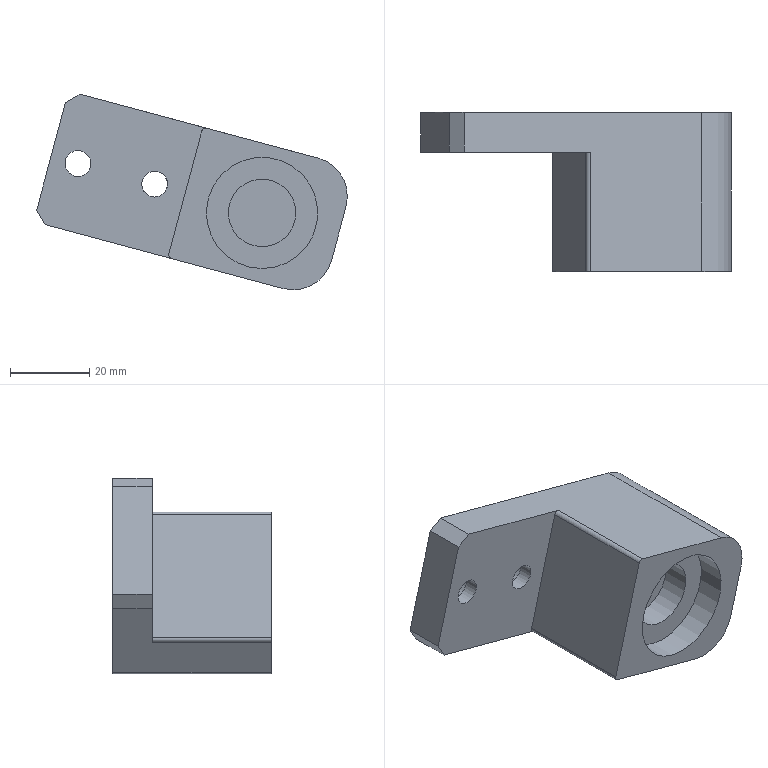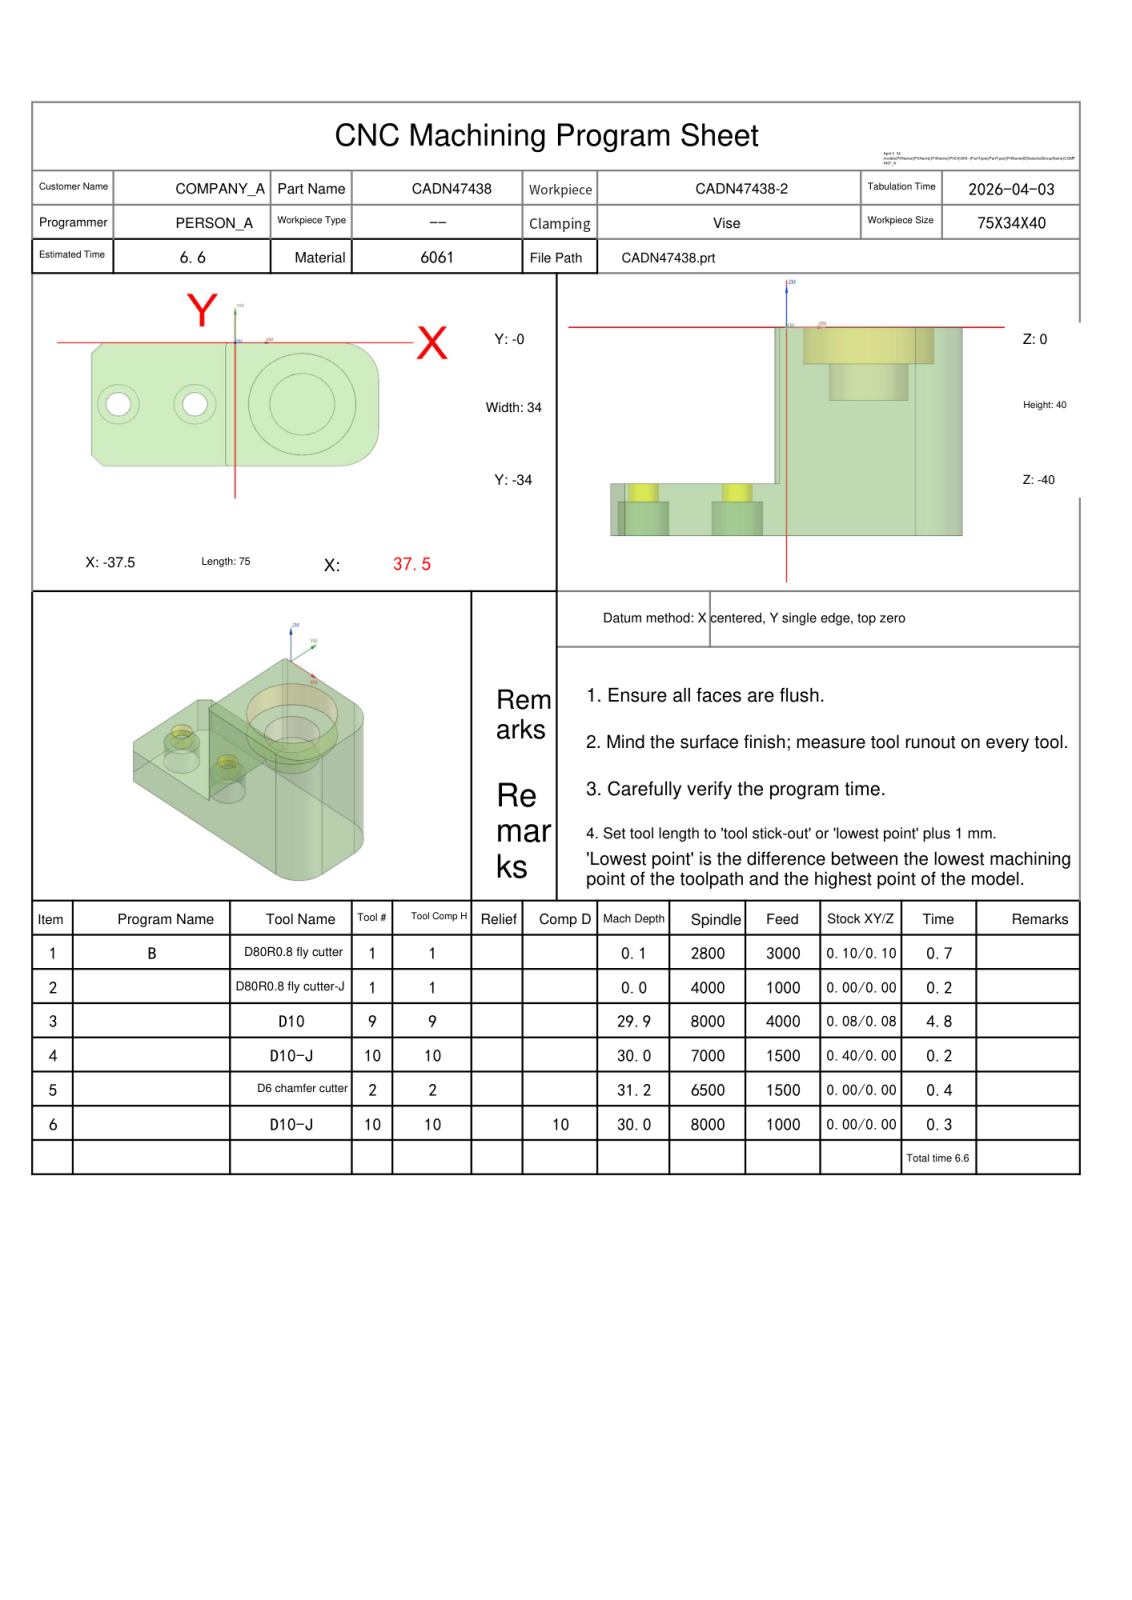NC program | NX | posted by the shop | part box 78.22 x 40 x 49.229 mm
Lines 109 to 1077 of 2756:
N3 T09 M06
(D10  D=10. R=0. H=09 ce=0.08 di=0.08)
G00 G90 G54 X17.5 Y-17. M03 S6000
G43 H09 Z20.
M08
Z.5
G03 X19.432 Y-18.482 I1.932 J.518 F2700.
X21.432 Y-16.482 I0.0 J2.
X21.364 Y-15.965 I-2. J0.0
X21.364 Y-15.965 Z.3 I-3.864 J-1.035 F3000.
X21.364 Y-15.965 Z.1 I-3.864 J-1.035
X21.364 Y-15.965 Z-.1 I-3.864 J-1.035
X21.364 Y-15.965 Z-.3 I-3.864 J-1.035
X21.364 Y-15.965 Z-.5 I-3.864 J-1.035
X21.364 Y-15.965 Z-.7 I-3.864 J-1.035
X21.364 Y-15.965 Z-.9 I-3.864 J-1.035
X21.364 Y-15.965 Z-1.1 I-3.864 J-1.035
X21.364 Y-15.965 Z-1.3 I-3.864 J-1.035
X21.364 Y-15.965 Z-1.5 I-3.864 J-1.035
X21.364 Y-15.965 Z-1.7 I-3.864 J-1.035
X21.364 Y-15.965 Z-1.9 I-3.864 J-1.035
X21.364 Y-15.965 Z-2.1 I-3.864 J-1.035
X21.364 Y-15.965 Z-2.3 I-3.864 J-1.035
X21.364 Y-15.965 Z-2.5 I-3.864 J-1.035
X21.364 Y-15.965 Z-2.7 I-3.864 J-1.035
X21.364 Y-15.965 Z-2.9 I-3.864 J-1.035
X21.364 Y-15.965 Z-3.1 I-3.864 J-1.035
X21.364 Y-15.965 Z-3.3 I-3.864 J-1.035
X21.364 Y-15.965 Z-3.5 I-3.864 J-1.035
X21.364 Y-15.965 Z-3.7 I-3.864 J-1.035
X21.364 Y-15.965 Z-3.9 I-3.864 J-1.035
X21.364 Y-15.965 Z-4.1 I-3.864 J-1.035
X21.364 Y-15.965 Z-4.3 I-3.864 J-1.035
X21.364 Y-15.965 Z-4.5 I-3.864 J-1.035
X21.364 Y-15.965 Z-4.7 I-3.864 J-1.035
X21.364 Y-15.965 Z-4.9 I-3.864 J-1.035
X21.364 Y-15.965 Z-5.1 I-3.864 J-1.035
X21.364 Y-15.965 Z-5.3 I-3.864 J-1.035
X21.364 Y-15.965 Z-5.5 I-3.864 J-1.035
X21.364 Y-15.965 Z-5.7 I-3.864 J-1.035
X21.364 Y-15.965 Z-5.9 I-3.864 J-1.035
X21.364 Y-15.965 Z-6.1 I-3.864 J-1.035
X21.364 Y-15.965 Z-6.3 I-3.864 J-1.035
X21.364 Y-15.965 Z-6.5 I-3.864 J-1.035
X21.364 Y-15.965 Z-6.7 I-3.864 J-1.035
X21.364 Y-15.965 Z-6.9 I-3.864 J-1.035
X20.017 Y-13.891 Z-6.92 I-3.864 J-1.035
X17.445 Y-12.981 I-2.572 J-3.176
X14.319 Y-14.434 I0.0 J-4.087
X13.34 Y-17.116 I3.183 J-2.681
X14.705 Y-20.197 I4.162 J0.0
X17.589 Y-21.311 I2.884 J3.177
X20.713 Y-19.962 I0.0 J4.291
X21.923 Y-16.912 I-3.238 J3.05
X20.583 Y-13.73 I-4.449 J0.0
X17.412 Y-12.438 I-3.171 J-3.246
X14.225 Y-13.746 I0.0 J-4.538
X12.827 Y-17.089 I3.298 J-3.343
X14.12 Y-20.324 I4.696 J0.0
X17.587 Y-21.812 I3.468 J3.297
X20.82 Y-20.555 I0.0 J4.785
X22.423 Y-16.911 I-3.339 J3.644
X21.186 Y-13.639 I-4.943 J0.0
X17.414 Y-11.938 I-3.772 J-3.331
X14.153 Y-13.137 I0.0 J-5.032
X12.326 Y-17.09 I3.363 J-3.953
X13.502 Y-20.379 I5.19 J0.0
X17.585 Y-22.312 I4.084 J3.346
X20.855 Y-21.178 I0.0 J5.279
X22.924 Y-16.91 I-3.367 J4.268
X21.818 Y-13.622 I-5.437 J0.0
X17.416 Y-11.438 I-4.401 J-3.342
X14.157 Y-12.501 I0.0 J-5.526
X11.825 Y-17.091 I3.352 J-4.59
X12.858 Y-20.358 I5.684 J0.0
X17.582 Y-22.813 I4.724 J3.318
X20.812 Y-21.824 I0.0 J5.773
X23.425 Y-16.909 I-3.318 J4.916
X22.471 Y-13.683 I-5.931 J0.0
X17.419 Y-10.937 I-5.051 J-3.275
X14.238 Y-11.846 I0.0 J-6.02
X11.325 Y-17.091 I3.264 J-5.245
X12.197 Y-20.257 I6.178 J0.0
X17.579 Y-23.313 I5.382 J3.212
X20.69 Y-22.486 I0.0 J6.267
X23.926 Y-16.909 I-3.189 J5.577
X23.137 Y-13.824 I-6.425 J0.0
X17.423 Y-10.437 I-5.714 J-3.128
X14.402 Y-11.18 I0.0 J-6.514
X10.824 Y-17.091 I3.094 J-5.911
X11.528 Y-20.074 I6.672 J0.0
X17.576 Y-23.812 I6.048 J3.023
X20.486 Y-23.154 I0.0 J6.761
X24.427 Y-16.909 I-2.978 J6.245
X23.807 Y-14.048 I-6.919 J0.0
X17.426 Y-9.938 I-6.381 J-2.898
X14.648 Y-10.512 I0.0 J-7.008
X10.323 Y-17.091 I2.841 J-6.579
X10.858 Y-19.808 I7.166 J0.0
X17.572 Y-24.312 I6.713 J2.752
X20.197 Y-23.82 I0.0 J7.255
X24.927 Y-16.91 I-2.683 J6.91
X24.474 Y-14.356 I-7.413 J0.0
X17.431 Y-9.438 I-7.043 J-2.584
X14.978 Y-9.85 I0.0 J-7.502
X9.822 Y-17.09 I2.504 J-7.239
X10.197 Y-19.458 I7.66 J0.0
X17.567 Y-24.811 I7.37 J2.396
X19.825 Y-24.475 I0.0 J7.749
X25.428 Y-16.911 I-2.303 J7.564
X25.127 Y-14.749 I-7.907 J0.0
X17.435 Y-8.939 I-7.692 J-2.186
X15.393 Y-9.204 I0.0 J-7.996
X9.322 Y-17.088 I2.082 J-7.883
X9.554 Y-19.022 I8.154 J0.0
X17.562 Y-25.31 I8.008 J1.956
X19.368 Y-25.11 I0.0 J8.243
X25.929 Y-16.913 I-1.84 J8.197
X25.758 Y-15.227 I-8.401 J0.0
X17.44 Y-8.441 I-8.318 J-1.704
X15.892 Y-8.583 I0.0 J-8.49
X8.821 Y-17.086 I1.577 J-8.503
X8.938 Y-18.504 I8.648 J0.0
X17.597 Y-25.842 I8.659 J1.439
X18.949 Y-25.737 I0.0 J8.777
X26.439 Y-16.988 I-1.365 J8.749
X26.357 Y-15.787 I-8.854 J0.0
X17.5 Y-8.06 I-8.857 J-1.213
X8.56 Y-17. I0.0 J-8.94
X17.5 Y-25.94 I8.94 J0.0
X26.44 Y-17. I0.0 J8.94
X26.276 Y-15.293 I-8.94 J0.0
X21.888 Y-11.677 I-4.388 J-.853
X17.418 Y-16.147 I0.0 J-4.47
X17.5 Y-17. I4.47 J0.0
G00 Z20.
G00 G90 X20.279 Y-18.949 M03 S8000
Z20.
Z-6.
G01 X20.47 Y-18.715 Z-6.016 F2000.
X20.864 Y-17.672 Z-6.074
X20.901 Y-16.557 Z-6.133
X20.667 Y-15.683 Z-6.18
X20.077 Y-14.737 Z-6.239
X19.215 Y-14.03 Z-6.297
X18.172 Y-13.636 Z-6.355
X17.057 Y-13.599 Z-6.414
X16.183 Y-13.833 Z-6.461
X15.237 Y-14.423 Z-6.52
X14.53 Y-15.285 Z-6.578
X14.136 Y-16.328 Z-6.637
X14.099 Y-17.443 Z-6.695
X14.333 Y-18.317 Z-6.743
X14.923 Y-19.263 Z-6.801
X15.785 Y-19.97 Z-6.859
X16.828 Y-20.364 Z-6.918
X17.943 Y-20.401 Z-6.976
X18.38 Y-20.284 Z-7.
G03 X20.784 Y-16.12 Z-7.062 I-.88 J3.284
X16.62 Y-13.716 Z-7.123 I-3.284 J-.88
X14.216 Y-17.88 Z-7.185 I.88 J-3.284
X18.38 Y-20.284 Z-7.246 I3.284 J.88
X20.784 Y-16.12 Z-7.308 I-.88 J3.284
X16.62 Y-13.716 Z-7.37 I-3.284 J-.88
X14.216 Y-17.88 Z-7.431 I.88 J-3.284
X18.38 Y-20.284 Z-7.493 I3.284 J.88
X20.784 Y-16.12 Z-7.554 I-.88 J3.284
X16.62 Y-13.716 Z-7.616 I-3.284 J-.88
X14.216 Y-17.88 Z-7.678 I.88 J-3.284
X18.38 Y-20.284 Z-7.739 I3.284 J.88
X20.784 Y-16.12 Z-7.801 I-.88 J3.284
X16.62 Y-13.716 Z-7.863 I-3.284 J-.88
X14.216 Y-17.88 Z-7.924 I.88 J-3.284
X18.38 Y-20.284 Z-7.986 I3.284 J.88
X20.784 Y-16.12 Z-8.047 I-.88 J3.284
X16.62 Y-13.716 Z-8.109 I-3.284 J-.88
X14.216 Y-17.88 Z-8.171 I.88 J-3.284
X18.38 Y-20.284 Z-8.232 I3.284 J.88
X20.784 Y-16.12 Z-8.294 I-.88 J3.284
X16.62 Y-13.716 Z-8.355 I-3.284 J-.88
X14.216 Y-17.88 Z-8.417 I.88 J-3.284
X18.38 Y-20.284 Z-8.479 I3.284 J.88
X20.784 Y-16.12 Z-8.54 I-.88 J3.284
X16.62 Y-13.716 Z-8.602 I-3.284 J-.88
X14.216 Y-17.88 Z-8.663 I.88 J-3.284
X18.38 Y-20.284 Z-8.725 I3.284 J.88
X20.784 Y-16.12 Z-8.787 I-.88 J3.284
X16.62 Y-13.716 Z-8.848 I-3.284 J-.88
X14.216 Y-17.88 Z-8.91 I.88 J-3.284
X18.38 Y-20.284 Z-8.971 I3.284 J.88
X20.784 Y-16.12 Z-9.033 I-.88 J3.284
X16.62 Y-13.716 Z-9.095 I-3.284 J-.88
X14.216 Y-17.88 Z-9.156 I.88 J-3.284
X18.38 Y-20.284 Z-9.218 I3.284 J.88
X20.784 Y-16.12 Z-9.279 I-.88 J3.284
X16.62 Y-13.716 Z-9.341 I-3.284 J-.88
X14.216 Y-17.88 Z-9.403 I.88 J-3.284
X18.38 Y-20.284 Z-9.464 I3.284 J.88
X20.784 Y-16.12 Z-9.526 I-.88 J3.284
X16.62 Y-13.716 Z-9.588 I-3.284 J-.88
X14.216 Y-17.88 Z-9.649 I.88 J-3.284
X18.38 Y-20.284 Z-9.711 I3.284 J.88
X20.784 Y-16.12 Z-9.772 I-.88 J3.284
X16.62 Y-13.716 Z-9.834 I-3.284 J-.88
X14.216 Y-17.88 Z-9.896 I.88 J-3.284
X18.38 Y-20.284 Z-9.957 I3.284 J.88
X20.784 Y-16.12 Z-10.019 I-.88 J3.284
X16.62 Y-13.716 Z-10.08 I-3.284 J-.88
X14.216 Y-17.88 Z-10.142 I.88 J-3.284
X18.38 Y-20.284 Z-10.204 I3.284 J.88
X20.784 Y-16.12 Z-10.265 I-.88 J3.284
X16.62 Y-13.716 Z-10.327 I-3.284 J-.88
X14.216 Y-17.88 Z-10.388 I.88 J-3.284
X18.38 Y-20.284 Z-10.45 I3.284 J.88
X20.784 Y-16.12 Z-10.512 I-.88 J3.284
X16.62 Y-13.716 Z-10.573 I-3.284 J-.88
X14.216 Y-17.88 Z-10.635 I.88 J-3.284
X18.38 Y-20.284 Z-10.696 I3.284 J.88
X20.784 Y-16.12 Z-10.758 I-.88 J3.284
X16.62 Y-13.716 Z-10.82 I-3.284 J-.88
X14.216 Y-17.88 Z-10.881 I.88 J-3.284
X18.38 Y-20.284 Z-10.943 I3.284 J.88
X20.784 Y-16.12 Z-11.004 I-.88 J3.284
X16.62 Y-13.716 Z-11.066 I-3.284 J-.88
X14.216 Y-17.88 Z-11.128 I.88 J-3.284
X18.38 Y-20.284 Z-11.189 I3.284 J.88
X20.784 Y-16.12 Z-11.251 I-.88 J3.284
X16.62 Y-13.716 Z-11.313 I-3.284 J-.88
X14.216 Y-17.88 Z-11.374 I.88 J-3.284
X18.38 Y-20.284 Z-11.436 I3.284 J.88
X20.784 Y-16.12 Z-11.497 I-.88 J3.284
X16.62 Y-13.716 Z-11.559 I-3.284 J-.88
X14.216 Y-17.88 Z-11.621 I.88 J-3.284
X18.38 Y-20.284 Z-11.682 I3.284 J.88
X20.784 Y-16.12 Z-11.744 I-.88 J3.284
X16.62 Y-13.716 Z-11.805 I-3.284 J-.88
X14.216 Y-17.88 Z-11.867 I.88 J-3.284
X18.38 Y-20.284 Z-11.929 I3.284 J.88
X20.784 Y-16.12 Z-11.99 I-.88 J3.284
X16.62 Y-13.716 Z-12.052 I-3.284 J-.88
X14.216 Y-17.88 Z-12.113 I.88 J-3.284
X18.38 Y-20.284 Z-12.175 I3.284 J.88
X20.784 Y-16.12 Z-12.237 I-.88 J3.284
X16.62 Y-13.716 Z-12.298 I-3.284 J-.88
X14.216 Y-17.88 Z-12.36 I.88 J-3.284
X18.38 Y-20.284 Z-12.421 I3.284 J.88
X20.784 Y-16.12 Z-12.483 I-.88 J3.284
X16.62 Y-13.716 Z-12.545 I-3.284 J-.88
X14.216 Y-17.88 Z-12.606 I.88 J-3.284
X18.38 Y-20.284 Z-12.668 I3.284 J.88
X20.784 Y-16.12 Z-12.729 I-.88 J3.284
X16.62 Y-13.716 Z-12.791 I-3.284 J-.88
X14.216 Y-17.88 Z-12.853 I.88 J-3.284
X18.38 Y-20.284 Z-12.914 I3.284 J.88
X20.784 Y-16.12 Z-12.976 I-.88 J3.284
X16.62 Y-13.716 Z-13.038 I-3.284 J-.88
X14.216 Y-17.88 Z-13.099 I.88 J-3.284
X18.38 Y-20.284 Z-13.161 I3.284 J.88
X20.784 Y-16.12 Z-13.222 I-.88 J3.284
X16.62 Y-13.716 Z-13.284 I-3.284 J-.88
X14.216 Y-17.88 Z-13.346 I.88 J-3.284
X18.38 Y-20.284 Z-13.407 I3.284 J.88
X20.784 Y-16.12 Z-13.469 I-.88 J3.284
X16.62 Y-13.716 Z-13.53 I-3.284 J-.88
X14.216 Y-17.88 Z-13.592 I.88 J-3.284
X18.38 Y-20.284 Z-13.654 I3.284 J.88
X20.784 Y-16.12 Z-13.715 I-.88 J3.284
X16.62 Y-13.716 Z-13.777 I-3.284 J-.88
X14.216 Y-17.88 Z-13.838 I.88 J-3.284
X18.38 Y-20.284 Z-13.9 I3.284 J.88
X20.9 Y-17. I-.88 J3.284
X17.5 Y-13.6 I-3.4 J0.0
X14.1 Y-17. I0.0 J-3.4
X17.5 Y-20.4 I3.4 J0.0
X18.38 Y-20.284 I0.0 J3.4
X18.759 Y-20.158 I-.88 J3.284
G01 Z-12.9
G00 Z20.
G00 G90 X-36.67 Y-41.997 M03 S8000
Z14.5
Z.902
G01 Z-.598 F4000.
X-37.222 Y-38.207
G02 X-37.6 Y-33. I35.722 J5.207
G01 Y-1.
G02 X-37.27 Y3.872 I36.1 J0.0
X-36.986 Y4.443 I.991 J-.135
G01 X-36.822 Y4.607
G02 X-36.116 Y4.9 I.707 J-.707
G01 X-30.454
G02 X-29.654 Y4.1 I0.0 J-.8
G01 X-29.666 Y3.962
G03 X-30.1 Y-1. I28.166 J-4.962
G01 Y-33.
G03 X-29.646 Y-38.078 I28.6 J0.0
X-28.662 Y-38.9 I.984 J.178
G01 X-22.67
G03 X-21.971 Y-38.2 I0.0 J.7
G01 X-21.991 Y-38.033
G02 X-22.6 Y-33. I20.491 J5.033
G01 Y-1.
G02 X-21.963 Y4.144 I21.1 J0.0
X-20.994 Y4.9 I.97 J-.244
G01 X-14.673
G02 X-14.074 Y4.3 I0.0 J-.6
X-14.117 Y4.076 I-.6 J0.0
G03 X-15.1 Y-1. I12.617 J-5.076
G01 Y-33.
G03 X-13.977 Y-38.412 I13.6 J0.0
X-13.246 Y-38.996 I.917 J.398
G01 X-3.49 Y-40.85
X-3.303 Y-40.867
G03 X-2.303 Y-39.867 I0.0 J1.
X-3.049 Y-38.9 I-1. J0.0
G02 X-7.6 Y-33. I1.549 J5.9
G01 Y-1.
G02 X-3.049 Y4.9 I6.1 J0.0
G01 X-.148 Y5.662
Y8.1
Z.902
G00 Z14.5
X-36.67 Y-41.997
Z.304
G01 Z-1.196
X-37.222 Y-38.207
G02 X-37.6 Y-33. I35.722 J5.207
G01 Y-1.
G02 X-37.27 Y3.872 I36.1 J0.0
X-36.986 Y4.443 I.991 J-.135
G01 X-36.822 Y4.607
G02 X-36.116 Y4.9 I.707 J-.707
G01 X-30.454
G02 X-29.654 Y4.1 I0.0 J-.8
G01 X-29.666 Y3.962
G03 X-30.1 Y-1. I28.166 J-4.962
G01 Y-33.
G03 X-29.646 Y-38.078 I28.6 J0.0
X-28.662 Y-38.9 I.984 J.178
G01 X-22.67
G03 X-21.971 Y-38.2 I0.0 J.7
G01 X-21.991 Y-38.033
G02 X-22.6 Y-33. I20.491 J5.033
G01 Y-1.
G02 X-21.963 Y4.144 I21.1 J0.0
X-20.994 Y4.9 I.97 J-.244
G01 X-14.673
G02 X-14.074 Y4.3 I0.0 J-.6
X-14.117 Y4.076 I-.6 J0.0
G03 X-15.1 Y-1. I12.617 J-5.076
G01 Y-33.
G03 X-13.977 Y-38.412 I13.6 J0.0
X-13.246 Y-38.996 I.917 J.398
G01 X-3.49 Y-40.85
X-3.303 Y-40.867
G03 X-2.303 Y-39.867 I0.0 J1.
X-3.049 Y-38.9 I-1. J0.0
G02 X-7.6 Y-33. I1.549 J5.9
G01 Y-1.
G02 X-3.049 Y4.9 I6.1 J0.0
G01 X-.148 Y5.662
Y8.1
Z.304
G00 Z14.5
X-36.67 Y-41.997
Z-.294
G01 Z-1.794
X-37.222 Y-38.207
G02 X-37.6 Y-33. I35.722 J5.207
G01 Y-1.
G02 X-37.27 Y3.872 I36.1 J0.0
X-36.986 Y4.443 I.991 J-.135
G01 X-36.822 Y4.607
G02 X-36.116 Y4.9 I.707 J-.707
G01 X-30.454
G02 X-29.654 Y4.1 I0.0 J-.8
G01 X-29.666 Y3.962
G03 X-30.1 Y-1. I28.166 J-4.962
G01 Y-33.
G03 X-29.646 Y-38.078 I28.6 J0.0
X-28.662 Y-38.9 I.984 J.178
G01 X-22.67
G03 X-21.971 Y-38.2 I0.0 J.7
G01 X-21.991 Y-38.033
G02 X-22.6 Y-33. I20.491 J5.033
G01 Y-1.
G02 X-21.963 Y4.144 I21.1 J0.0
X-20.994 Y4.9 I.97 J-.244
G01 X-14.673
G02 X-14.074 Y4.3 I0.0 J-.6
X-14.117 Y4.076 I-.6 J0.0
G03 X-15.1 Y-1. I12.617 J-5.076
G01 Y-33.
G03 X-13.977 Y-38.412 I13.6 J0.0
X-13.246 Y-38.996 I.917 J.398
G01 X-3.49 Y-40.85
X-3.303 Y-40.867
G03 X-2.303 Y-39.867 I0.0 J1.
X-3.049 Y-38.9 I-1. J0.0
G02 X-7.6 Y-33. I1.549 J5.9
G01 Y-1.
G02 X-3.049 Y4.9 I6.1 J0.0
G01 X-.148 Y5.662
Y8.1
Z-.294
G00 Z14.5
X-36.67 Y-41.997
Z-.892
G01 Z-2.392
X-37.222 Y-38.207
G02 X-37.6 Y-33. I35.722 J5.207
G01 Y-1.
G02 X-37.27 Y3.872 I36.1 J0.0
X-36.986 Y4.443 I.991 J-.135
G01 X-36.822 Y4.607
G02 X-36.116 Y4.9 I.707 J-.707
G01 X-30.454
G02 X-29.654 Y4.1 I0.0 J-.8
G01 X-29.666 Y3.962
G03 X-30.1 Y-1. I28.166 J-4.962
G01 Y-33.
G03 X-29.646 Y-38.078 I28.6 J0.0
X-28.662 Y-38.9 I.984 J.178
G01 X-22.67
G03 X-21.971 Y-38.2 I0.0 J.7
G01 X-21.991 Y-38.033
G02 X-22.6 Y-33. I20.491 J5.033
G01 Y-1.
G02 X-21.963 Y4.144 I21.1 J0.0
X-20.994 Y4.9 I.97 J-.244
G01 X-14.673
G02 X-14.074 Y4.3 I0.0 J-.6
X-14.117 Y4.076 I-.6 J0.0
G03 X-15.1 Y-1. I12.617 J-5.076
G01 Y-33.
G03 X-13.977 Y-38.412 I13.6 J0.0
X-13.246 Y-38.996 I.917 J.398
G01 X-3.49 Y-40.85
X-3.303 Y-40.867
G03 X-2.303 Y-39.867 I0.0 J1.
X-3.049 Y-38.9 I-1. J0.0
G02 X-7.6 Y-33. I1.549 J5.9
G01 Y-1.
G02 X-3.049 Y4.9 I6.1 J0.0
G01 X-.148 Y5.662
Y8.1
Z-.892
G00 Z14.5
X-36.67 Y-41.997
Z-1.49
G01 Z-2.99
X-37.222 Y-38.207
G02 X-37.6 Y-33. I35.722 J5.207
G01 Y-1.
G02 X-37.27 Y3.872 I36.1 J0.0
X-36.986 Y4.443 I.991 J-.135
G01 X-36.822 Y4.607
G02 X-36.116 Y4.9 I.707 J-.707
G01 X-30.454
G02 X-29.654 Y4.1 I0.0 J-.8
G01 X-29.666 Y3.962
G03 X-30.1 Y-1. I28.166 J-4.962
G01 Y-33.
G03 X-29.646 Y-38.078 I28.6 J0.0
X-28.662 Y-38.9 I.984 J.178
G01 X-22.67
G03 X-21.971 Y-38.2 I0.0 J.7
G01 X-21.991 Y-38.033
G02 X-22.6 Y-33. I20.491 J5.033
G01 Y-1.
G02 X-21.963 Y4.144 I21.1 J0.0
X-20.994 Y4.9 I.97 J-.244
G01 X-14.673
G02 X-14.074 Y4.3 I0.0 J-.6
X-14.117 Y4.076 I-.6 J0.0
G03 X-15.1 Y-1. I12.617 J-5.076
G01 Y-33.
G03 X-13.977 Y-38.412 I13.6 J0.0
X-13.246 Y-38.996 I.917 J.398
G01 X-3.49 Y-40.85
X-3.303 Y-40.867
G03 X-2.303 Y-39.867 I0.0 J1.
X-3.049 Y-38.9 I-1. J0.0
G02 X-7.6 Y-33. I1.549 J5.9
G01 Y-1.
G02 X-3.049 Y4.9 I6.1 J0.0
G01 X-.148 Y5.662
Y8.1
Z-1.49
G00 Z14.5
X-36.67 Y-41.997
Z-2.088
G01 Z-3.588
X-37.222 Y-38.207
G02 X-37.6 Y-33. I35.722 J5.207
G01 Y-1.
G02 X-37.27 Y3.872 I36.1 J0.0
X-36.986 Y4.443 I.991 J-.135
G01 X-36.822 Y4.607
G02 X-36.116 Y4.9 I.707 J-.707
G01 X-30.454
G02 X-29.654 Y4.1 I0.0 J-.8
G01 X-29.666 Y3.962
G03 X-30.1 Y-1. I28.166 J-4.962
G01 Y-33.
G03 X-29.646 Y-38.078 I28.6 J0.0
X-28.662 Y-38.9 I.984 J.178
G01 X-22.67
G03 X-21.971 Y-38.2 I0.0 J.7
G01 X-21.991 Y-38.033
G02 X-22.6 Y-33. I20.491 J5.033
G01 Y-1.
G02 X-21.963 Y4.144 I21.1 J0.0
X-20.994 Y4.9 I.97 J-.244
G01 X-14.673
G02 X-14.074 Y4.3 I0.0 J-.6
X-14.117 Y4.076 I-.6 J0.0
G03 X-15.1 Y-1. I12.617 J-5.076
G01 Y-33.
G03 X-13.977 Y-38.412 I13.6 J0.0
X-13.246 Y-38.996 I.917 J.398
G01 X-3.49 Y-40.85
X-3.303 Y-40.867
G03 X-2.303 Y-39.867 I0.0 J1.
X-3.049 Y-38.9 I-1. J0.0
G02 X-7.6 Y-33. I1.549 J5.9
G01 Y-1.
G02 X-3.049 Y4.9 I6.1 J0.0
G01 X-.148 Y5.662
Y8.1
Z-2.088
G00 Z14.5
X-36.67 Y-41.997
Z-2.686
G01 Z-4.186
X-37.222 Y-38.207
G02 X-37.6 Y-33. I35.722 J5.207
G01 Y-1.
G02 X-37.27 Y3.872 I36.1 J0.0
X-36.986 Y4.443 I.991 J-.135
G01 X-36.822 Y4.607
G02 X-36.116 Y4.9 I.707 J-.707
G01 X-30.454
G02 X-29.654 Y4.1 I0.0 J-.8
G01 X-29.666 Y3.962
G03 X-30.1 Y-1. I28.166 J-4.962
G01 Y-33.
G03 X-29.646 Y-38.078 I28.6 J0.0
X-28.662 Y-38.9 I.984 J.178
G01 X-22.67
G03 X-21.971 Y-38.2 I0.0 J.7
G01 X-21.991 Y-38.033
G02 X-22.6 Y-33. I20.491 J5.033
G01 Y-1.
G02 X-21.963 Y4.144 I21.1 J0.0
X-20.994 Y4.9 I.97 J-.244
G01 X-14.673
G02 X-14.074 Y4.3 I0.0 J-.6
X-14.117 Y4.076 I-.6 J0.0
G03 X-15.1 Y-1. I12.617 J-5.076
G01 Y-33.
G03 X-13.977 Y-38.412 I13.6 J0.0
X-13.246 Y-38.996 I.917 J.398
G01 X-3.49 Y-40.85
X-3.303 Y-40.867
G03 X-2.303 Y-39.867 I0.0 J1.
X-3.049 Y-38.9 I-1. J0.0
G02 X-7.6 Y-33. I1.549 J5.9
G01 Y-1.
G02 X-3.049 Y4.9 I6.1 J0.0
G01 X-.148 Y5.662
Y8.1
Z-2.686
G00 Z14.5
X-36.67 Y-41.997
Z-3.284
G01 Z-4.784
X-37.222 Y-38.207
G02 X-37.6 Y-33. I35.722 J5.207
G01 Y-1.
G02 X-37.27 Y3.872 I36.1 J0.0
X-36.986 Y4.443 I.991 J-.135
G01 X-36.822 Y4.607
G02 X-36.116 Y4.9 I.707 J-.707
G01 X-30.454
G02 X-29.654 Y4.1 I0.0 J-.8
G01 X-29.666 Y3.962
G03 X-30.1 Y-1. I28.166 J-4.962
G01 Y-33.
G03 X-29.646 Y-38.078 I28.6 J0.0
X-28.662 Y-38.9 I.984 J.178
G01 X-22.67
G03 X-21.971 Y-38.2 I0.0 J.7
G01 X-21.991 Y-38.033
G02 X-22.6 Y-33. I20.491 J5.033
G01 Y-1.
G02 X-21.963 Y4.144 I21.1 J0.0
X-20.994 Y4.9 I.97 J-.244
G01 X-14.673
G02 X-14.074 Y4.3 I0.0 J-.6
X-14.117 Y4.076 I-.6 J0.0
G03 X-15.1 Y-1. I12.617 J-5.076
G01 Y-33.
G03 X-13.977 Y-38.412 I13.6 J0.0
X-13.246 Y-38.996 I.917 J.398
G01 X-3.49 Y-40.85
X-3.303 Y-40.867
G03 X-2.303 Y-39.867 I0.0 J1.
X-3.049 Y-38.9 I-1. J0.0
G02 X-7.6 Y-33. I1.549 J5.9
G01 Y-1.
G02 X-3.049 Y4.9 I6.1 J0.0
G01 X-.148 Y5.662
Y8.1
Z-3.284
G00 Z14.5
X-36.67 Y-41.997
Z-3.882
G01 Z-5.382
X-37.222 Y-38.207
G02 X-37.6 Y-33. I35.722 J5.207
G01 Y-1.
G02 X-37.27 Y3.872 I36.1 J0.0
X-36.986 Y4.443 I.991 J-.135
G01 X-36.822 Y4.607
G02 X-36.116 Y4.9 I.707 J-.707
G01 X-30.454
G02 X-29.654 Y4.1 I0.0 J-.8
G01 X-29.666 Y3.962
G03 X-30.1 Y-1. I28.166 J-4.962
G01 Y-33.
G03 X-29.646 Y-38.078 I28.6 J0.0
X-28.662 Y-38.9 I.984 J.178
G01 X-22.67
G03 X-21.971 Y-38.2 I0.0 J.7
G01 X-21.991 Y-38.033
G02 X-22.6 Y-33. I20.491 J5.033
G01 Y-1.
G02 X-21.963 Y4.144 I21.1 J0.0
X-20.994 Y4.9 I.97 J-.244
G01 X-14.673
G02 X-14.074 Y4.3 I0.0 J-.6
X-14.117 Y4.076 I-.6 J0.0
G03 X-15.1 Y-1. I12.617 J-5.076
G01 Y-33.
G03 X-13.977 Y-38.412 I13.6 J0.0
X-13.246 Y-38.996 I.917 J.398
G01 X-3.49 Y-40.85
X-3.303 Y-40.867
G03 X-2.303 Y-39.867 I0.0 J1.
X-3.049 Y-38.9 I-1. J0.0
G02 X-7.6 Y-33. I1.549 J5.9
G01 Y-1.
G02 X-3.049 Y4.9 I6.1 J0.0
G01 X-.148 Y5.662
Y8.1
Z-3.882
G00 Z14.5
X-36.67 Y-41.997
Z-4.48
G01 Z-5.98
X-37.222 Y-38.207
G02 X-37.6 Y-33. I35.722 J5.207
G01 Y-1.
G02 X-37.27 Y3.872 I36.1 J0.0
X-36.986 Y4.443 I.991 J-.135
G01 X-36.822 Y4.607
G02 X-36.116 Y4.9 I.707 J-.707
G01 X-30.454
G02 X-29.654 Y4.1 I0.0 J-.8
G01 X-29.666 Y3.962
G03 X-30.1 Y-1. I28.166 J-4.962
G01 Y-33.
G03 X-29.646 Y-38.078 I28.6 J0.0
X-28.662 Y-38.9 I.984 J.178
G01 X-22.67
G03 X-21.971 Y-38.2 I0.0 J.7
G01 X-21.991 Y-38.033
G02 X-22.6 Y-33. I20.491 J5.033
G01 Y-1.
G02 X-21.963 Y4.144 I21.1 J0.0
X-20.994 Y4.9 I.97 J-.244
G01 X-14.673
G02 X-14.074 Y4.3 I0.0 J-.6
X-14.117 Y4.076 I-.6 J0.0
G03 X-15.1 Y-1. I12.617 J-5.076
G01 Y-33.
G03 X-13.977 Y-38.412 I13.6 J0.0
X-13.246 Y-38.996 I.917 J.398
G01 X-3.49 Y-40.85
X-3.303 Y-40.867
G03 X-2.303 Y-39.867 I0.0 J1.
X-3.049 Y-38.9 I-1. J0.0
G02 X-7.6 Y-33. I1.549 J5.9
G01 Y-1.
G02 X-3.049 Y4.9 I6.1 J0.0
G01 X-.148 Y5.662
Y8.1
Z-4.48
G00 Z14.5
X-36.67 Y-41.997
Z-5.078
G01 Z-6.578
X-37.222 Y-38.207
G02 X-37.6 Y-33. I35.722 J5.207
G01 Y-1.
G02 X-37.27 Y3.872 I36.1 J0.0
X-36.986 Y4.443 I.991 J-.135
G01 X-36.822 Y4.607
G02 X-36.116 Y4.9 I.707 J-.707
G01 X-30.454
G02 X-29.654 Y4.1 I0.0 J-.8
G01 X-29.666 Y3.962
G03 X-30.1 Y-1. I28.166 J-4.962
G01 Y-33.
G03 X-29.646 Y-38.078 I28.6 J0.0
X-28.662 Y-38.9 I.984 J.178
G01 X-22.67
G03 X-21.971 Y-38.2 I0.0 J.7
G01 X-21.991 Y-38.033
G02 X-22.6 Y-33. I20.491 J5.033
G01 Y-1.
G02 X-21.963 Y4.144 I21.1 J0.0
X-20.994 Y4.9 I.97 J-.244
G01 X-14.673
G02 X-14.074 Y4.3 I0.0 J-.6
X-14.117 Y4.076 I-.6 J0.0
G03 X-15.1 Y-1. I12.617 J-5.076
G01 Y-33.
G03 X-13.977 Y-38.412 I13.6 J0.0
X-13.246 Y-38.996 I.917 J.398
G01 X-3.49 Y-40.85
X-3.303 Y-40.867
G03 X-2.303 Y-39.867 I0.0 J1.
X-3.049 Y-38.9 I-1. J0.0
G02 X-7.6 Y-33. I1.549 J5.9
G01 Y-1.
G02 X-3.049 Y4.9 I6.1 J0.0
G01 X-.148 Y5.662
Y8.1
Z-5.078
G00 Z14.5
X-36.67 Y-41.997
Z-5.676
G01 Z-7.176
X-37.222 Y-38.207
G02 X-37.6 Y-33. I35.722 J5.207
G01 Y-1.
G02 X-37.27 Y3.872 I36.1 J0.0
X-36.986 Y4.443 I.991 J-.135
G01 X-36.822 Y4.607
G02 X-36.116 Y4.9 I.707 J-.707
G01 X-30.454
G02 X-29.654 Y4.1 I0.0 J-.8
G01 X-29.666 Y3.962
G03 X-30.1 Y-1. I28.166 J-4.962
G01 Y-33.
G03 X-29.646 Y-38.078 I28.6 J0.0
X-28.662 Y-38.9 I.984 J.178
G01 X-22.67
G03 X-21.971 Y-38.2 I0.0 J.7
G01 X-21.991 Y-38.033
G02 X-22.6 Y-33. I20.491 J5.033
G01 Y-1.
G02 X-21.963 Y4.144 I21.1 J0.0
X-20.994 Y4.9 I.97 J-.244
G01 X-14.673
G02 X-14.074 Y4.3 I0.0 J-.6
X-14.117 Y4.076 I-.6 J0.0
G03 X-15.1 Y-1. I12.617 J-5.076
G01 Y-33.
G03 X-13.977 Y-38.412 I13.6 J0.0
X-13.246 Y-38.996 I.917 J.398
G01 X-3.49 Y-40.85
X-3.303 Y-40.867
G03 X-2.303 Y-39.867 I0.0 J1.
X-3.049 Y-38.9 I-1. J0.0
G02 X-7.6 Y-33. I1.549 J5.9
G01 Y-1.
G02 X-3.049 Y4.9 I6.1 J0.0
G01 X-.148 Y5.662
Y8.1
Z-5.676
G00 Z14.5
X-36.67 Y-41.997
Z-6.274
G01 Z-7.774
X-37.222 Y-38.207
G02 X-37.6 Y-33. I35.722 J5.207
G01 Y-1.
G02 X-37.27 Y3.872 I36.1 J0.0
X-36.986 Y4.443 I.991 J-.135
G01 X-36.822 Y4.607
G02 X-36.116 Y4.9 I.707 J-.707
G01 X-30.454
G02 X-29.654 Y4.1 I0.0 J-.8
G01 X-29.666 Y3.962
G03 X-30.1 Y-1. I28.166 J-4.962
G01 Y-33.
G03 X-29.646 Y-38.078 I28.6 J0.0
X-28.662 Y-38.9 I.984 J.178
G01 X-22.67
G03 X-21.971 Y-38.2 I0.0 J.7
G01 X-21.991 Y-38.033
G02 X-22.6 Y-33. I20.491 J5.033
G01 Y-1.
G02 X-21.963 Y4.144 I21.1 J0.0
X-20.994 Y4.9 I.97 J-.244
G01 X-14.673
G02 X-14.074 Y4.3 I0.0 J-.6
X-14.117 Y4.076 I-.6 J0.0
G03 X-15.1 Y-1. I12.617 J-5.076
G01 Y-33.
G03 X-13.977 Y-38.412 I13.6 J0.0
X-13.246 Y-38.996 I.917 J.398
G01 X-3.49 Y-40.85
X-3.303 Y-40.867
G03 X-2.303 Y-39.867 I0.0 J1.
X-3.049 Y-38.9 I-1. J0.0
G02 X-7.6 Y-33. I1.549 J5.9
G01 Y-1.
G02 X-3.049 Y4.9 I6.1 J0.0
G01 X-.148 Y5.662
Y8.1
Z-6.274
G00 Z14.5
X-36.67 Y-41.997
Z-6.872
G01 Z-8.372
X-37.222 Y-38.207
G02 X-37.6 Y-33. I35.722 J5.207
G01 Y-1.
G02 X-37.27 Y3.872 I36.1 J0.0
X-36.986 Y4.443 I.991 J-.135
G01 X-36.822 Y4.607
G02 X-36.116 Y4.9 I.707 J-.707
G01 X-30.454
G02 X-29.654 Y4.1 I0.0 J-.8
G01 X-29.666 Y3.962
G03 X-30.1 Y-1. I28.166 J-4.962
G01 Y-33.
G03 X-29.646 Y-38.078 I28.6 J0.0
X-28.662 Y-38.9 I.984 J.178
G01 X-22.67
G03 X-21.971 Y-38.2 I0.0 J.7
G01 X-21.991 Y-38.033
G02 X-22.6 Y-33. I20.491 J5.033
G01 Y-1.
G02 X-21.963 Y4.144 I21.1 J0.0
X-20.994 Y4.9 I.97 J-.244
G01 X-14.673
G02 X-14.074 Y4.3 I0.0 J-.6
X-14.117 Y4.076 I-.6 J0.0
G03 X-15.1 Y-1. I12.617 J-5.076
G01 Y-33.
G03 X-13.977 Y-38.412 I13.6 J0.0
X-13.246 Y-38.996 I.917 J.398
G01 X-3.49 Y-40.85
X-3.303 Y-40.867
G03 X-2.303 Y-39.867 I0.0 J1.
X-3.049 Y-38.9 I-1. J0.0
G02 X-7.6 Y-33. I1.549 J5.9
G01 Y-1.
G02 X-3.049 Y4.9 I6.1 J0.0
G01 X-.148 Y5.662
Y8.1
Z-6.872
G00 Z14.5
X-36.67 Y-41.997
Z-7.47
G01 Z-8.97
X-37.222 Y-38.207
G02 X-37.6 Y-33. I35.722 J5.207
G01 Y-1.
G02 X-37.27 Y3.872 I36.1 J0.0
X-36.986 Y4.443 I.991 J-.135
G01 X-36.822 Y4.607
G02 X-36.116 Y4.9 I.707 J-.707
G01 X-30.454
G02 X-29.654 Y4.1 I0.0 J-.8
G01 X-29.666 Y3.962
G03 X-30.1 Y-1. I28.166 J-4.962
G01 Y-33.
G03 X-29.646 Y-38.078 I28.6 J0.0
X-28.662 Y-38.9 I.984 J.178
G01 X-22.67
G03 X-21.971 Y-38.2 I0.0 J.7
G01 X-21.991 Y-38.033
G02 X-22.6 Y-33. I20.491 J5.033
G01 Y-1.
G02 X-21.963 Y4.144 I21.1 J0.0
X-20.994 Y4.9 I.97 J-.244
G01 X-14.673
G02 X-14.074 Y4.3 I0.0 J-.6
X-14.117 Y4.076 I-.6 J0.0
G03 X-15.1 Y-1. I12.617 J-5.076
G01 Y-33.
G03 X-13.977 Y-38.412 I13.6 J0.0
X-13.246 Y-38.996 I.917 J.398
G01 X-3.49 Y-40.85
X-3.303 Y-40.867
G03 X-2.303 Y-39.867 I0.0 J1.
X-3.049 Y-38.9 I-1. J0.0
G02 X-7.6 Y-33. I1.549 J5.9
G01 Y-1.
G02 X-3.049 Y4.9 I6.1 J0.0
G01 X-.148 Y5.662
Y8.1
Z-7.47
G00 Z14.5
X-36.67 Y-41.997
Z-8.068
G01 Z-9.568
X-37.222 Y-38.207
G02 X-37.6 Y-33. I35.722 J5.207
G01 Y-1.
G02 X-37.27 Y3.872 I36.1 J0.0
X-36.986 Y4.443 I.991 J-.135
G01 X-36.822 Y4.607
G02 X-36.116 Y4.9 I.707 J-.707
G01 X-30.454
G02 X-29.654 Y4.1 I0.0 J-.8
G01 X-29.666 Y3.962
G03 X-30.1 Y-1. I28.166 J-4.962
G01 Y-33.
G03 X-29.646 Y-38.078 I28.6 J0.0
X-28.662 Y-38.9 I.984 J.178
G01 X-22.67
G03 X-21.971 Y-38.2 I0.0 J.7
G01 X-21.991 Y-38.033
G02 X-22.6 Y-33. I20.491 J5.033
G01 Y-1.
G02 X-21.963 Y4.144 I21.1 J0.0
X-20.994 Y4.9 I.97 J-.244
G01 X-14.673
G02 X-14.074 Y4.3 I0.0 J-.6
X-14.117 Y4.076 I-.6 J0.0
G03 X-15.1 Y-1. I12.617 J-5.076
G01 Y-33.
G03 X-13.977 Y-38.412 I13.6 J0.0
X-13.246 Y-38.996 I.917 J.398
G01 X-3.49 Y-40.85
X-3.303 Y-40.867
G03 X-2.303 Y-39.867 I0.0 J1.
X-3.049 Y-38.9 I-1. J0.0
G02 X-7.6 Y-33. I1.549 J5.9
G01 Y-1.
G02 X-3.049 Y4.9 I6.1 J0.0
G01 X-.148 Y5.662
Y8.1
Z-8.068
G00 Z14.5
X-36.67 Y-41.997
Z-8.666
G01 Z-10.166
X-37.222 Y-38.207
G02 X-37.6 Y-33. I35.722 J5.207
G01 Y-1.
G02 X-37.27 Y3.872 I36.1 J0.0
X-36.986 Y4.443 I.991 J-.135
G01 X-36.822 Y4.607
G02 X-36.116 Y4.9 I.707 J-.707
G01 X-30.454
G02 X-29.654 Y4.1 I0.0 J-.8
G01 X-29.666 Y3.962
G03 X-30.1 Y-1. I28.166 J-4.962
G01 Y-33.
G03 X-29.646 Y-38.078 I28.6 J0.0
X-28.662 Y-38.9 I.984 J.178
G01 X-22.67